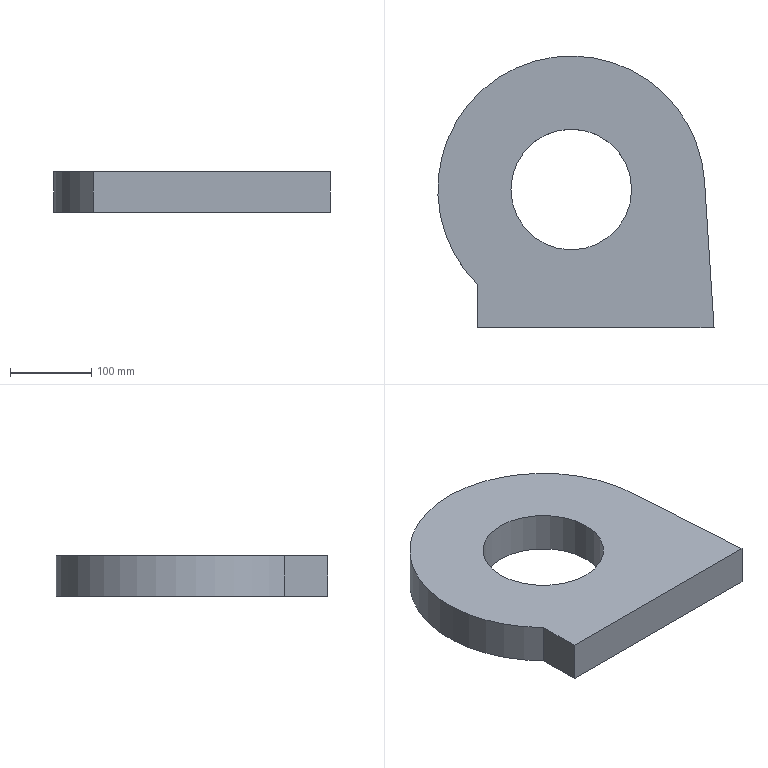Part | NX | features 底座(默认<按焊接>) 2 | 1 solid | 7 faces | box 339.407 x 334 x 50 mm | volume 3868356 mm3 | plane 5 | cylinder 2 | commonest cylinder face diameters 148.4 x1 328 x1
STEP:
#1=CARTESIAN_POINT('',(1576.181,817.42,-892.));
#2=VERTEX_POINT('',#1);
#3=CARTESIAN_POINT('',(1855.485,944.347,-892.));
#4=VERTEX_POINT('',#3);
#5=CARTESIAN_POINT('',(1691.831,933.7,-892.));
#6=DIRECTION('',(0.,0.,-1.));
#7=DIRECTION('',(-1.,0.,0.));
#8=AXIS2_PLACEMENT_3D('',#5,#6,#7);
#9=CIRCLE('',#8,164.);
#10=EDGE_CURVE('',#2,#4,#9,.T.);
#11=ORIENTED_EDGE('',*,*,#10,.F.);
#12=CARTESIAN_POINT('',(1576.181,817.42,-842.));
#13=VERTEX_POINT('',#12);
#14=CARTESIAN_POINT('',(1576.181,817.42,-842.));
#15=DIRECTION('',(0.,0.,-1.));
#16=VECTOR('',#15,1000.);
#17=LINE('',#14,#16);
#18=EDGE_CURVE('',#13,#2,#17,.T.);
#19=ORIENTED_EDGE('',*,*,#18,.F.);
#20=CARTESIAN_POINT('',(1855.485,944.347,-842.));
#21=VERTEX_POINT('',#20);
#22=CARTESIAN_POINT('',(1691.831,933.7,-842.));
#23=DIRECTION('',(0.,0.,-1.));
#24=DIRECTION('',(-1.,0.,0.));
#25=AXIS2_PLACEMENT_3D('',#22,#23,#24);
#26=CIRCLE('',#25,164.);
#27=EDGE_CURVE('',#13,#21,#26,.T.);
#28=ORIENTED_EDGE('',*,*,#27,.T.);
#29=CARTESIAN_POINT('',(1855.485,944.347,-842.));
#30=DIRECTION('',(0.,0.,-1.));
#31=VECTOR('',#30,1000.);
#32=LINE('',#29,#31);
#33=EDGE_CURVE('',#21,#4,#32,.T.);
#34=ORIENTED_EDGE('',*,*,#33,.T.);
#35=EDGE_LOOP('',(#11,#19,#28,#34));
#36=FACE_BOUND('',#35,.T.);
#37=CARTESIAN_POINT('',(1691.831,933.7,-842.));
#38=DIRECTION('',(0.,0.,-1.));
#39=DIRECTION('',(1.,0.,0.));
#40=AXIS2_PLACEMENT_3D('',#37,#38,#39);
#41=CYLINDRICAL_SURFACE('',#40,164.);
#42=ADVANCED_FACE('',(#36),#41,.T.);
#43=CARTESIAN_POINT('',(1867.238,763.7,-892.));
#44=VERTEX_POINT('',#43);
#45=CARTESIAN_POINT('',(1855.485,944.347,-892.));
#46=DIRECTION('',(0.06492,-0.9979,0.));
#47=VECTOR('',#46,1000.);
#48=LINE('',#45,#47);
#49=EDGE_CURVE('',#4,#44,#48,.T.);
#50=ORIENTED_EDGE('',*,*,#49,.F.);
#51=ORIENTED_EDGE('',*,*,#33,.F.);
#52=CARTESIAN_POINT('',(1867.238,763.7,-842.));
#53=VERTEX_POINT('',#52);
#54=CARTESIAN_POINT('',(1855.485,944.347,-842.));
#55=DIRECTION('',(0.06492,-0.9979,0.));
#56=VECTOR('',#55,1000.);
#57=LINE('',#54,#56);
#58=EDGE_CURVE('',#21,#53,#57,.T.);
#59=ORIENTED_EDGE('',*,*,#58,.T.);
#60=CARTESIAN_POINT('',(1867.238,763.7,-842.));
#61=DIRECTION('',(0.,0.,-1.));
#62=VECTOR('',#61,1000.);
#63=LINE('',#60,#62);
#64=EDGE_CURVE('',#53,#44,#63,.T.);
#65=ORIENTED_EDGE('',*,*,#64,.T.);
#66=EDGE_LOOP('',(#50,#51,#59,#65));
#67=FACE_BOUND('',#66,.T.);
#68=CARTESIAN_POINT('',(1855.485,944.347,-842.));
#69=DIRECTION('',(-0.9979,-0.06492,0.));
#70=DIRECTION('',(0.06492,-0.9979,0.));
#71=AXIS2_PLACEMENT_3D('',#68,#69,#70);
#72=PLANE('',#71);
#73=ADVANCED_FACE('',(#67),#72,.F.);
#74=CARTESIAN_POINT('',(1576.181,763.7,-892.));
#75=VERTEX_POINT('',#74);
#76=CARTESIAN_POINT('',(1867.238,763.7,-892.));
#77=DIRECTION('',(-1.,0.,0.));
#78=VECTOR('',#77,1000.);
#79=LINE('',#76,#78);
#80=EDGE_CURVE('',#44,#75,#79,.T.);
#81=ORIENTED_EDGE('',*,*,#80,.F.);
#82=ORIENTED_EDGE('',*,*,#64,.F.);
#83=CARTESIAN_POINT('',(1576.181,763.7,-842.));
#84=VERTEX_POINT('',#83);
#85=CARTESIAN_POINT('',(1867.238,763.7,-842.));
#86=DIRECTION('',(-1.,0.,0.));
#87=VECTOR('',#86,1000.);
#88=LINE('',#85,#87);
#89=EDGE_CURVE('',#53,#84,#88,.T.);
#90=ORIENTED_EDGE('',*,*,#89,.T.);
#91=CARTESIAN_POINT('',(1576.181,763.7,-842.));
#92=DIRECTION('',(0.,0.,-1.));
#93=VECTOR('',#92,1000.);
#94=LINE('',#91,#93);
#95=EDGE_CURVE('',#84,#75,#94,.T.);
#96=ORIENTED_EDGE('',*,*,#95,.T.);
#97=EDGE_LOOP('',(#81,#82,#90,#96));
#98=FACE_BOUND('',#97,.T.);
#99=CARTESIAN_POINT('',(1867.238,763.7,-842.));
#100=DIRECTION('',(0.,1.,0.));
#101=DIRECTION('',(0.,0.,-1.));
#102=AXIS2_PLACEMENT_3D('',#99,#100,#101);
#103=PLANE('',#102);
#104=ADVANCED_FACE('',(#98),#103,.F.);
#105=CARTESIAN_POINT('',(1576.181,817.42,-892.));
#106=DIRECTION('',(0.,1.,0.));
#107=VECTOR('',#106,1000.);
#108=LINE('',#105,#107);
#109=EDGE_CURVE('',#75,#2,#108,.T.);
#110=ORIENTED_EDGE('',*,*,#109,.F.);
#111=ORIENTED_EDGE('',*,*,#95,.F.);
#112=CARTESIAN_POINT('',(1576.181,817.42,-842.));
#113=DIRECTION('',(0.,1.,0.));
#114=VECTOR('',#113,1000.);
#115=LINE('',#112,#114);
#116=EDGE_CURVE('',#84,#13,#115,.T.);
#117=ORIENTED_EDGE('',*,*,#116,.T.);
#118=ORIENTED_EDGE('',*,*,#18,.T.);
#119=EDGE_LOOP('',(#110,#111,#117,#118));
#120=FACE_BOUND('',#119,.T.);
#121=CARTESIAN_POINT('',(1576.181,817.42,-842.));
#122=DIRECTION('',(1.,0.,0.));
#123=DIRECTION('',(0.,0.,1.));
#124=AXIS2_PLACEMENT_3D('',#121,#122,#123);
#125=PLANE('',#124);
#126=ADVANCED_FACE('',(#120),#125,.F.);
#127=CARTESIAN_POINT('',(1617.631,933.7,-842.));
#128=VERTEX_POINT('',#127);
#129=CARTESIAN_POINT('',(1691.831,933.7,-842.));
#130=DIRECTION('',(0.,0.,-1.));
#131=DIRECTION('',(-1.,0.,0.));
#132=AXIS2_PLACEMENT_3D('',#129,#130,#131);
#133=CIRCLE('',#132,74.2);
#134=EDGE_CURVE('',#128,#128,#133,.T.);
#135=ORIENTED_EDGE('',*,*,#134,.T.);
#136=EDGE_LOOP('',(#135));
#137=FACE_BOUND('',#136,.T.);
#138=ORIENTED_EDGE('',*,*,#27,.F.);
#139=ORIENTED_EDGE('',*,*,#116,.F.);
#140=ORIENTED_EDGE('',*,*,#89,.F.);
#141=ORIENTED_EDGE('',*,*,#58,.F.);
#142=EDGE_LOOP('',(#138,#139,#140,#141));
#143=FACE_BOUND('',#142,.T.);
#144=CARTESIAN_POINT('',(1691.831,933.7,-842.));
#145=DIRECTION('',(0.,0.,1.));
#146=DIRECTION('',(-1.,0.,0.));
#147=AXIS2_PLACEMENT_3D('',#144,#145,#146);
#148=PLANE('',#147);
#149=ADVANCED_FACE('',(#137,#143),#148,.T.);
#150=CARTESIAN_POINT('',(1617.631,933.7,-892.));
#151=VERTEX_POINT('',#150);
#152=CARTESIAN_POINT('',(1691.831,933.7,-892.));
#153=DIRECTION('',(0.,0.,-1.));
#154=DIRECTION('',(-1.,0.,0.));
#155=AXIS2_PLACEMENT_3D('',#152,#153,#154);
#156=CIRCLE('',#155,74.2);
#157=EDGE_CURVE('',#151,#151,#156,.T.);
#158=ORIENTED_EDGE('',*,*,#157,.F.);
#159=EDGE_LOOP('',(#158));
#160=FACE_BOUND('',#159,.T.);
#161=ORIENTED_EDGE('',*,*,#10,.T.);
#162=ORIENTED_EDGE('',*,*,#49,.T.);
#163=ORIENTED_EDGE('',*,*,#80,.T.);
#164=ORIENTED_EDGE('',*,*,#109,.T.);
#165=EDGE_LOOP('',(#161,#162,#163,#164));
#166=FACE_BOUND('',#165,.T.);
#167=CARTESIAN_POINT('',(1691.831,933.7,-892.));
#168=DIRECTION('',(0.,0.,1.));
#169=DIRECTION('',(-1.,0.,0.));
#170=AXIS2_PLACEMENT_3D('',#167,#168,#169);
#171=PLANE('',#170);
#172=ADVANCED_FACE('',(#160,#166),#171,.F.);
#173=ORIENTED_EDGE('',*,*,#134,.F.);
#174=EDGE_LOOP('',(#173));
#175=FACE_BOUND('',#174,.T.);
#176=ORIENTED_EDGE('',*,*,#157,.T.);
#177=EDGE_LOOP('',(#176));
#178=FACE_BOUND('',#177,.T.);
#179=CARTESIAN_POINT('',(1691.831,933.7,-396.));
#180=DIRECTION('',(0.,0.,-1.));
#181=DIRECTION('',(1.,0.,0.));
#182=AXIS2_PLACEMENT_3D('',#179,#180,#181);
#183=CYLINDRICAL_SURFACE('',#182,74.2);
#184=ADVANCED_FACE('',(#175,#178),#183,.F.);
#185=CLOSED_SHELL('',(#42,#73,#104,#126,#149,#172,#184));
#186=MANIFOLD_SOLID_BREP('',#185);
#187=(LENGTH_UNIT()NAMED_UNIT(*)SI_UNIT(.MILLI.,.METRE.));
#188=UNCERTAINTY_MEASURE_WITH_UNIT(LENGTH_MEASURE(0.00001),#187,'','');
#189=(NAMED_UNIT(*)PLANE_ANGLE_UNIT()SI_UNIT($,.RADIAN.));
#190=(NAMED_UNIT(*)SI_UNIT($,.STERADIAN.)SOLID_ANGLE_UNIT());
#191=(GEOMETRIC_REPRESENTATION_CONTEXT(3)GLOBAL_UNCERTAINTY_ASSIGNED_CONTEXT((#188))GLOBAL_UNIT_ASSIGNED_CONTEXT((#187,#189,#190))REPRESENTATION_CONTEXT('',''));
#192=ADVANCED_BREP_SHAPE_REPRESENTATION('',(#186),#191);